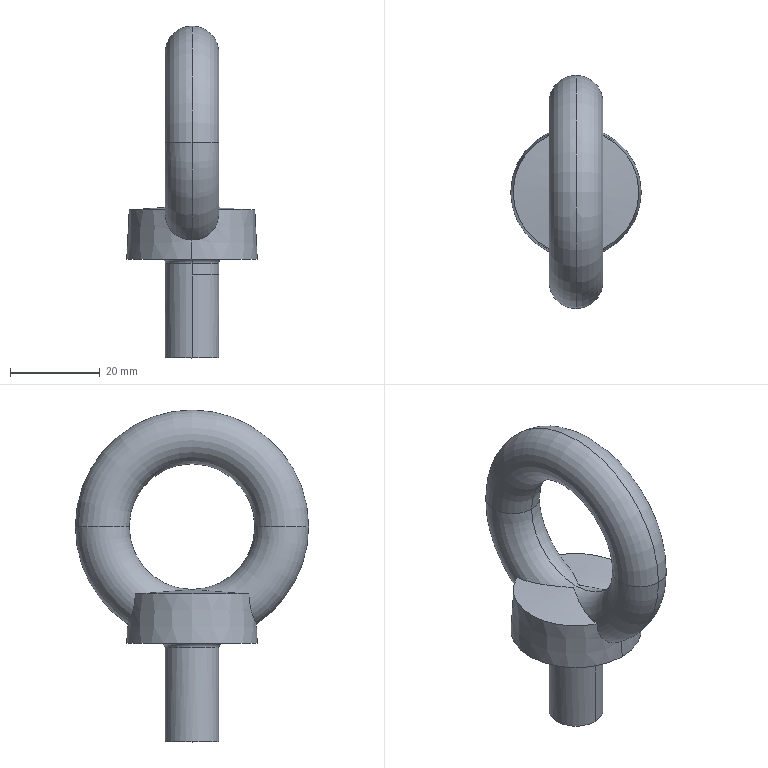Part | NX | features solid 2 | 1 solid | 18 faces | box 29.1 x 52 x 74 mm | volume 21178 mm3 | torus 6 | cylinder 4 | cone 4 | plane 2 | sphere 2 | commonest cylinder face diameters 12 x4